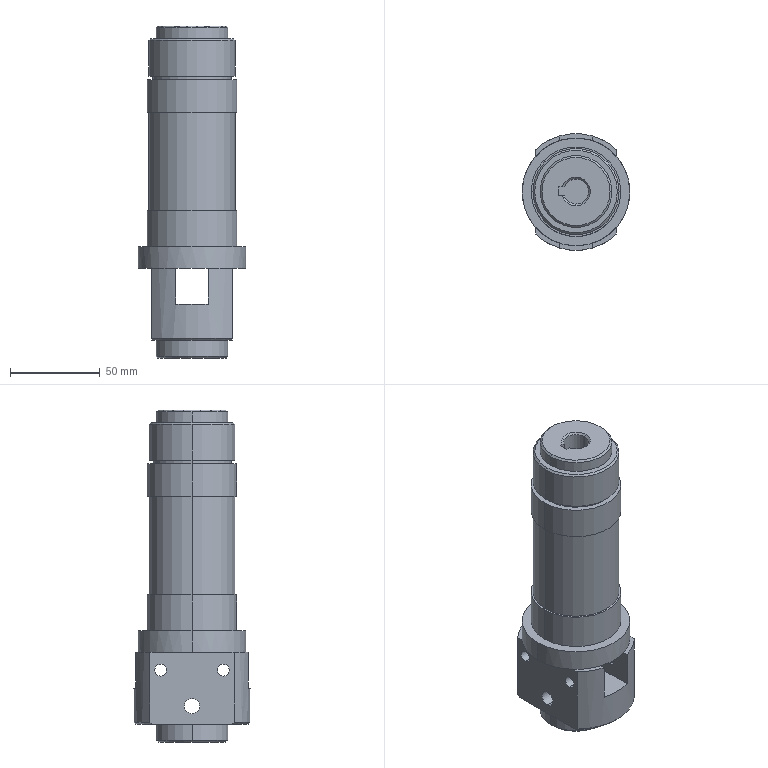Part | STEP file | YCD14007A-08.03.07.03 Shaft (Motor) | 1 solid | 68 faces | box 60 x 65 x 185 mm | volume 341019 mm3 | cylinder 32 | plane 26 | cone 10 | commonest cylinder face diameters 6.6 x8 40 x4 48 x4 50 x4 8.5 x2 14 x2